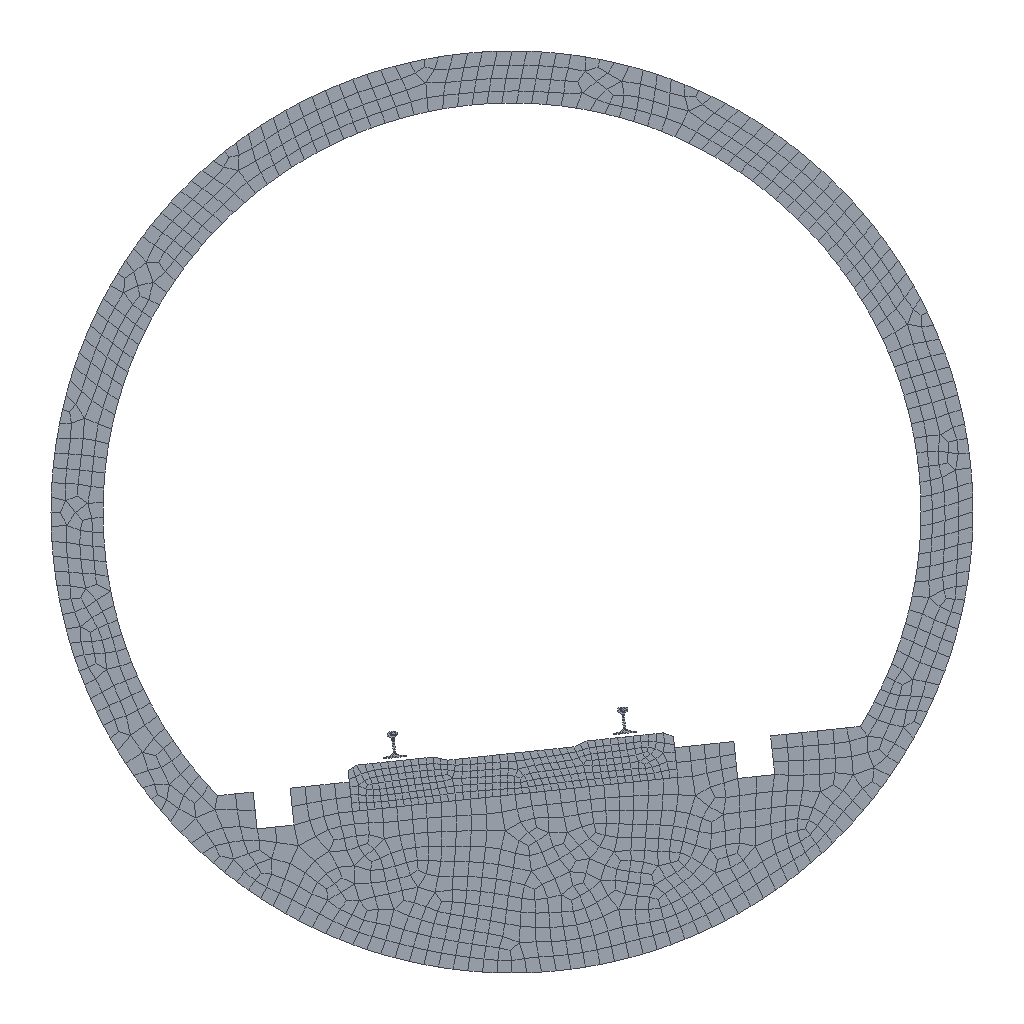Simulation study | abaqus
Set-up summary:
category,name,step,type,value,unit,region
solver,abaqus
solver,version,,,Abaqus/Standard 2020
units,not stated in the deck,,not stated
analysis,deck,,transient,transient
load_step,Step-1,Step-1,transient
load_step,requested,,,1
mesh,nodes,,,1882
mesh,elements,,,1560
element_type,CPS4R,,plane,1560
load,load commands in deck,,count,2
bc,support commands in deck,,count,1
material,CONCRETE,,in results
material,GUIZHEN,,in results
material,STEEL,,in results
check,setup vs results,,match,"per instance, exact: element labels, types and connectivity; labels of the nodes the elements use; coordinates of those nodes at SINGLE_PRECISION in 3 of 4 instance(s)"
Abaqus input file, long lists of numbers shortened:
*Heading
** Job name: Job-1 Model name: Model-1
** Generated by: Abaqus/CAE 2020
*Preprint, echo=NO, model=NO, history=NO, contact=NO
**
** PARTS
**
*Part, name=guizhen
*Node
      1,       -1037.,         913.
      2,       -1098.,        882.5
** (334 more lines like these left out)
*Element, type=CPS4R
  1, 331,  99,   1,  11
  2, 219, 261, 122, 120
** (284 more lines like these left out)
*Nset, nset=Set-1, generate
   1,  336,    1
*Elset, elset=Set-1, generate
   1,  286,    1
*Nset, nset=Set-2, generate
   1,  336,    1
*Elset, elset=Set-2, generate
   1,  286,    1
** Section: Section-3
*Solid Section, elset=Set-2, material=guizhen
,
*End Part
**
*Part, name=rail
*Node
      1,    -406.188,     360.812
      2,    -406.188,       364.75
** (159 more lines like these left out)
*Element, type=CPS4R
  1,  47,  48, 116, 117
  2,   3,   4,  97, 122
** (117 more lines like these left out)
*Nset, nset=Set-1, generate
   1,  161,    1
*Elset, elset=Set-1, generate
   1,  119,    1
*Nset, nset=Set-2, generate
   1,  161,    1
*Elset, elset=Set-2, generate
   1,  119,    1
** Section: Section-2
*Solid Section, elset=Set-2, material=steel
,
*End Part
**
*Part, name=structure
*Node
      1,   2478.045,  -1192.389
      2,   2554.355,  -1018.71
** (1222 more lines like these left out)
*Element, type=CPS4R
   1,  608,  582,  815,  240
   2,  553,  847, 1170,  239
** (1034 more lines like these left out)
*Nset, nset=Set-1, generate
    1,  1224,     1
*Elset, elset=Set-1, generate
    1,  1036,     1
*Nset, nset=Set-2, generate
    1,  1224,     1
*Elset, elset=Set-2, generate
    1,  1036,     1
** Section: Section-1
*Solid Section, elset=Set-2, material=concrete
,
*End Part
**
**
** ASSEMBLY
**
*Assembly, name=Assembly
**
*Instance, name=guizhen-1, part=guizhen
7804.25, -2501.585,           0.
7804.25, -2501.585,           0., 7804.25, -2501.585, 1., 6.
*End Instance
**
*Instance, name=rail-1, part=rail
7354.92, -1851.68,           0.
7354.92, -1851.68,           0., 7354.92, -1851.68, 1., 6.
*End Instance
**
*Instance, name=structure-1, part=structure
       7720.,           0.,           0.
*End Instance
**
*Instance, name=rail-1-lin-2-1, part=rail
8901.899, -1689.086,           0.
8901.899, -1689.086,           0., 8901.899, -1689.086, 1., 6.
*End Instance
**
*Node
      1,   6935.326,  -1674.883,           0.
*Node
      2,   6871.67,  -1648.302,           0.
*Node
      3,   6993.064,  -1635.542,           0.
*Node
      4,   8482.305,  -1512.289,           0.
*Node
      5,   8418.649,  -1485.708,           0.
*Node
      6,   8540.043,  -1472.948,           0.
*Node
      7,   8422.305,  -1518.289,           0.
*Node
      8,   8542.305,  -1506.289,           0.
*Node
      9,   6995.326,  -1667.883,           0.
*Node
     10,   6875.326,  -1680.883,           0.
*Node
     11,   6930.74,  -1474.075,           0.
*Node
     12,   8446.34,  -1314.779,           0.
*Nset, nset=Set-12
  2,  3,  5,  6,  7,  8,  9, 10
*Nset, nset=Set-13, instance=structure-1
  71,  72,  73,  74,  75,  76,  77,  78,  79,  80,  81,  82,  83,  84,  85,  86
  87,  88,  89,  90,  91,  92,  93,  94,  95,  96,  97,  98,  99, 100, 101, 102
** (11 more lines like these left out)
*Elset, elset=Set-13, instance=structure-1
  11,  12,  13,  19,  20,  46,  49,  58,  59,  65,  66,  67,  70,  71,  75,  76
 130, 131, 133, 138, 139, 146, 147, 148, 153, 167, 168, 169, 178, 181, 182, 183
** (11 more lines like these left out)
*Nset, nset=Set-14, instance=rail-1
 36,
*Nset, nset=Set-15, instance=rail-1
 36,
*Nset, nset=Set-16, instance=rail-1
 36,
*Nset, nset=Set-17
 11,
*Nset, nset=Set-18, generate
  7,  10,   1
*Nset, nset=Set-22
 2, 3
*Nset, nset=Set-23
 2, 3, 5, 6
*Nset, nset=Set-25
 12,
*Nset, nset=m_Set-13, instance=rail-1
 36,
*Nset, nset=m_Set-15
 11,
*Nset, nset=m_Set-18
 2,
*Nset, nset=m_Set-19
 3,
*Nset, nset=m_Set-20
 5,
*Nset, nset=m_Set-21
 6,
*Nset, nset=m_Set-24
 12,
*Nset, nset=m_Set-26
  9, 10
*Nset, nset=m_Set-27
 7, 8
*Nset, nset=m_Set-28
 10,
*Nset, nset=m_Set-29
 9,
*Nset, nset=m_Set-30
 7,
*Nset, nset=m_Set-31
 8,
*Nset, nset=m_Set-32
 10,
*Nset, nset=m_Set-33
 9,
*Nset, nset=m_Set-34
 7,
*Nset, nset=m_Set-35
 8,
*Elset, elset=_m_Surf-1_S4, internal, instance=structure-1
  26,  28,  36, 100, 418, 419
*Elset, elset=_m_Surf-1_S3, internal, instance=structure-1
 29, 39
*Elset, elset=_m_Surf-1_S2, internal, instance=structure-1
  41,  54, 109, 119, 123, 124, 322, 415, 416, 417, 733, 734, 735, 736, 737, 745
 746, 866
*Surface, type=ELEMENT, name=m_Surf-1
_m_Surf-1_S4, S4
_m_Surf-1_S3, S3
_m_Surf-1_S2, S2
*Elset, elset=_m_Surf-3_S4, internal, instance=structure-1
  26,  28,  36, 100, 418, 419
*Elset, elset=_m_Surf-3_S3, internal, instance=structure-1
 29, 39
*Elset, elset=_m_Surf-3_S2, internal, instance=structure-1
  41,  54, 109, 119, 123, 124, 322, 415, 416, 417, 733, 734, 735, 736, 737, 745
 746, 866
*Surface, type=ELEMENT, name=m_Surf-3
_m_Surf-3_S4, S4
_m_Surf-3_S3, S3
_m_Surf-3_S2, S2
*Elset, elset=_m_Surf-5_S1, internal, instance=rail-1-lin-2-1
  6,  8, 10, 15, 54, 91
*Elset, elset=_m_Surf-5_S4, internal, instance=rail-1-lin-2-1
  7, 13, 52
*Elset, elset=_m_Surf-5_S3, internal, instance=rail-1-lin-2-1
   9,  50,  90,  93, 112
*Elset, elset=_m_Surf-5_S2, internal, instance=rail-1-lin-2-1
  46,  66, 106
*Surface, type=ELEMENT, name=m_Surf-5
_m_Surf-5_S1, S1
_m_Surf-5_S4, S4
_m_Surf-5_S2, S2
_m_Surf-5_S3, S3
*Elset, elset=_m_Surf-7_S1, internal, instance=rail-1
  6,  8, 10, 15, 54, 91
*Elset, elset=_m_Surf-7_S4, internal, instance=rail-1
  7, 13, 52
*Elset, elset=_m_Surf-7_S3, internal, instance=rail-1
   9,  50,  90,  93, 112
*Elset, elset=_m_Surf-7_S2, internal, instance=rail-1
  46,  66, 106
*Surface, type=ELEMENT, name=m_Surf-7
_m_Surf-7_S1, S1
_m_Surf-7_S4, S4
_m_Surf-7_S2, S2
_m_Surf-7_S3, S3
*Elset, elset=_m_Surf-9_S2, internal, instance=guizhen-1
 9,
*Elset, elset=_m_Surf-9_S1, internal, instance=guizhen-1
 13,
*Elset, elset=_m_Surf-9_S3, internal, instance=guizhen-1
  92, 285
*Elset, elset=_m_Surf-9_S4, internal, instance=guizhen-1
 117,
*Surface, type=ELEMENT, name=m_Surf-9
_m_Surf-9_S2, S2
_m_Surf-9_S1, S1
_m_Surf-9_S4, S4
_m_Surf-9_S3, S3
*Elset, elset=_m_Surf-11_S4, internal, instance=guizhen-1
  11,  12,  18,  22,  23,  35,  37,  40,  42,  49,  51,  54,  62,  70,  74,  79
  83,  89,  91,  95,  97,  99, 108, 118, 126, 129
*Elset, elset=_m_Surf-11_S2, internal, instance=guizhen-1
  13,  16,  24,  30,  43,  47,  53,  55, 101, 102, 106, 110, 111, 112, 120, 121
 124, 128
*Surface, type=ELEMENT, name=m_Surf-11
_m_Surf-11_S4, S4
_m_Surf-11_S2, S2
*Elset, elset=_m_Surf-13_S3, internal, instance=guizhen-1
 55,
*Elset, elset=_m_Surf-13_S1, internal, instance=guizhen-1
 132, 133, 238
*Elset, elset=_m_Surf-13_S2, internal, instance=guizhen-1
 279,
*Surface, type=ELEMENT, name=m_Surf-13
_m_Surf-13_S3, S3
_m_Surf-13_S1, S1
_m_Surf-13_S2, S2
*Elset, elset=_m_Surf-20_S4, internal, instance=structure-1
  26,  28,  36, 100, 418, 419
*Elset, elset=_m_Surf-20_S3, internal, instance=structure-1
 29, 39
*Elset, elset=_m_Surf-20_S2, internal, instance=structure-1
  41,  54, 109, 119, 123, 124, 322, 415, 416, 417, 733, 734, 735, 736, 737, 745
 746, 866
*Surface, type=ELEMENT, name=m_Surf-20
_m_Surf-20_S4, S4
_m_Surf-20_S3, S3
_m_Surf-20_S2, S2
*Elset, elset=_s_Surf-1_S2, internal, instance=guizhen-1
   9, 279
*Elset, elset=_s_Surf-1_S1, internal, instance=guizhen-1
  13, 132, 133, 238
*Elset, elset=_s_Surf-1_S3, internal, instance=guizhen-1
  55,  92, 285
*Elset, elset=_s_Surf-1_S4, internal, instance=guizhen-1
 117,
*Surface, type=ELEMENT, name=s_Surf-1
_s_Surf-1_S2, S2
_s_Surf-1_S1, S1
_s_Surf-1_S4, S4
_s_Surf-1_S3, S3
*Elset, elset=_s_Surf-3_S2, internal, instance=guizhen-1
   9,  13,  16,  24,  30,  43,  47,  53,  55, 101, 102, 106, 110, 111, 112, 120
 121, 124, 128, 279
*Elset, elset=_s_Surf-3_S1, internal, instance=guizhen-1
  13, 132, 133, 238
*Elset, elset=_s_Surf-3_S3, internal, instance=guizhen-1
  55,  92, 285
*Elset, elset=_s_Surf-3_S4, internal, instance=guizhen-1
  11,  12,  18,  22,  23,  35,  37,  40,  42,  49,  51,  54,  62,  70,  74,  79
  83,  89,  91,  95,  97,  99, 108, 117, 118, 126, 129
*Surface, type=ELEMENT, name=s_Surf-3
_s_Surf-3_S2, S2
_s_Surf-3_S1, S1
_s_Surf-3_S4, S4
_s_Surf-3_S3, S3
*Elset, elset=_s_Surf-5_S3, internal, instance=guizhen-1
   7,  46,  48,  58,  59,  63,  66, 130
*Elset, elset=_s_Surf-5_S1, internal, instance=guizhen-1
  45, 153
*Surface, type=ELEMENT, name=s_Surf-5
_s_Surf-5_S3, S3
_s_Surf-5_S1, S1
*Elset, elset=_s_Surf-7_S3, internal, instance=guizhen-1
   4,  10,  15,  86,  90,  98, 158
*Elset, elset=_s_Surf-7_S1, internal, instance=guizhen-1
  85, 152, 160
*Surface, type=ELEMENT, name=s_Surf-7
_s_Surf-7_S3, S3
_s_Surf-7_S1, S1
*Elset, elset=_s_Surf-9_S4, internal, instance=structure-1
 28,
*Elset, elset=_s_Surf-9_S3, internal, instance=structure-1
 29,
*Surface, type=ELEMENT, name=s_Surf-9
_s_Surf-9_S4, S4
_s_Surf-9_S3, S3
*Elset, elset=_s_Surf-11_S4, internal, instance=structure-1
  26, 100, 418, 419
*Elset, elset=_s_Surf-11_S2, internal, instance=structure-1
  41,  54, 109, 119, 123, 124, 322, 415, 416, 417, 733, 734, 735, 736, 737, 745
 746, 866
*Surface, type=ELEMENT, name=s_Surf-11
_s_Surf-11_S4, S4
_s_Surf-11_S2, S2
*Elset, elset=_s_Surf-13_S4, internal, instance=structure-1
 36,
*Elset, elset=_s_Surf-13_S3, internal, instance=structure-1
 39,
*Surface, type=ELEMENT, name=s_Surf-13
_s_Surf-13_S4, S4
_s_Surf-13_S3, S3
*Elset, elset=_s_Surf-15_S2, internal, instance=rail-1
 30, 31, 84
*Elset, elset=_s_Surf-15_S1, internal, instance=rail-1
 35, 82
*Elset, elset=_s_Surf-15_S3, internal, instance=rail-1
 95,
*Surface, type=ELEMENT, name=s_Surf-15
_s_Surf-15_S2, S2
_s_Surf-15_S1, S1
_s_Surf-15_S3, S3
*Elset, elset=_s_Surf-16_S3, internal, instance=rail-1
 73, 74
*Elset, elset=_s_Surf-16_S1, internal, instance=rail-1
  14,  44, 113
*Elset, elset=_s_Surf-16_S4, internal, instance=rail-1
  14, 114
*Elset, elset=_s_Surf-16_S2, internal, instance=rail-1
 67,
*Surface, type=ELEMENT, name=s_Surf-16
_s_Surf-16_S3, S3
_s_Surf-16_S1, S1
_s_Surf-16_S4, S4
_s_Surf-16_S2, S2
*Elset, elset=_s_Surf-17_S1, internal, instance=rail-1
 102,
*Elset, elset=_s_Surf-17_S4, internal, instance=rail-1
  12,  56, 103
*Elset, elset=_s_Surf-17_S2, internal, instance=rail-1
 11, 57, 70
*Surface, type=ELEMENT, name=s_Surf-17
_s_Surf-17_S1, S1
_s_Surf-17_S4, S4
_s_Surf-17_S2, S2
*Elset, elset=_s_Surf-18_S3, internal, instance=rail-1-lin-2-1
 73, 74
*Elset, elset=_s_Surf-18_S1, internal, instance=rail-1-lin-2-1
  14,  44, 113
*Elset, elset=_s_Surf-18_S4, internal, instance=rail-1-lin-2-1
  14, 114
*Elset, elset=_s_Surf-18_S2, internal, instance=rail-1-lin-2-1
 67,
*Surface, type=ELEMENT, name=s_Surf-18
_s_Surf-18_S3, S3
_s_Surf-18_S1, S1
_s_Surf-18_S4, S4
_s_Surf-18_S2, S2
*Elset, elset=_s_Surf-19_S1, internal, instance=rail-1-lin-2-1
 102,
*Elset, elset=_s_Surf-19_S4, internal, instance=rail-1-lin-2-1
  12,  56, 103
*Elset, elset=_s_Surf-19_S2, internal, instance=rail-1-lin-2-1
 11, 57, 70
*Surface, type=ELEMENT, name=s_Surf-19
_s_Surf-19_S1, S1
_s_Surf-19_S4, S4
_s_Surf-19_S2, S2
*Elset, elset=_s_Surf-20_S2, internal, instance=guizhen-1
   9,  13,  16,  24,  30,  43,  47,  53,  55, 101, 102, 106, 110, 111, 112, 120
 121, 124, 128, 279
*Elset, elset=_s_Surf-20_S1, internal, instance=guizhen-1
  13, 132, 133, 238
*Elset, elset=_s_Surf-20_S3, internal, instance=guizhen-1
  55,  92, 285
*Elset, elset=_s_Surf-20_S4, internal, instance=guizhen-1
  11,  12,  18,  22,  23,  35,  37,  40,  42,  49,  51,  54,  62,  70,  74,  79
  83,  89,  91,  95,  97,  99, 108, 117, 118, 126, 129
*Surface, type=ELEMENT, name=s_Surf-20
_s_Surf-20_S2, S2
_s_Surf-20_S1, S1
_s_Surf-20_S4, S4
_s_Surf-20_S3, S3
*Elset, elset=_s_Surf-22_S2, internal, instance=rail-1-lin-2-1
 30, 83, 84
*Elset, elset=_s_Surf-22_S3, internal, instance=rail-1-lin-2-1
 64, 95
*Elset, elset=_s_Surf-22_S1, internal, instance=rail-1-lin-2-1
 115,
*Elset, elset=_s_Surf-22_S4, internal, instance=rail-1-lin-2-1
 25,
*Surface, type=ELEMENT, name=s_Surf-22
_s_Surf-22_S2, S2
_s_Surf-22_S3, S3
_s_Surf-22_S4, S4
_s_Surf-22_S1, S1
*Elset, elset=_s_Surf-23_S3, internal, instance=guizhen-1
   4,  10,  15,  86,  90,  98, 158
*Elset, elset=_s_Surf-23_S1, internal, instance=guizhen-1
  85, 152, 160
*Surface, type=ELEMENT, name=s_Surf-23
_s_Surf-23_S3, S3
_s_Surf-23_S1, S1
*Elset, elset=_s_Surf-24_S3, internal, instance=guizhen-1
   7,  46,  48,  58,  59,  63,  66, 130
*Elset, elset=_s_Surf-24_S1, internal, instance=guizhen-1
  45, 153
*Surface, type=ELEMENT, name=s_Surf-24
_s_Surf-24_S3, S3
_s_Surf-24_S1, S1
*Elset, elset=_s_Surf-25_S3, internal, instance=guizhen-1
   4,  10,  15,  86,  90,  98, 158
*Elset, elset=_s_Surf-25_S1, internal, instance=guizhen-1
  85, 152, 160
*Surface, type=ELEMENT, name=s_Surf-25
_s_Surf-25_S3, S3
_s_Surf-25_S1, S1
*Elset, elset=_s_Surf-26_S3, internal, instance=guizhen-1
   7,  46,  48,  58,  59,  63,  66, 130
*Elset, elset=_s_Surf-26_S1, internal, instance=guizhen-1
  45, 153
*Surface, type=ELEMENT, name=s_Surf-26
_s_Surf-26_S3, S3
_s_Surf-26_S1, S1
*Elset, elset=_s_Surf-27_S3, internal, instance=guizhen-1
   7,  46,  48,  58,  59,  63,  66, 130
*Elset, elset=_s_Surf-27_S1, internal, instance=guizhen-1
  45, 153
*Surface, type=ELEMENT, name=s_Surf-27
_s_Surf-27_S3, S3
_s_Surf-27_S1, S1
*Elset, elset=_s_Surf-28_S3, internal, instance=guizhen-1
 1,
*Elset, elset=_s_Surf-28_S2, internal, instance=guizhen-1
 285,
*Surface, type=ELEMENT, name=s_Surf-28
_s_Surf-28_S3, S3
_s_Surf-28_S2, S2
*Elset, elset=_s_Surf-29_S3, internal, instance=guizhen-1
 21, 84
*Surface, type=ELEMENT, name=s_Surf-29
_s_Surf-29_S3, S3
*Elset, elset=_s_Surf-30_S1, internal, instance=guizhen-1
 8,
*Elset, elset=_s_Surf-30_S3, internal, instance=guizhen-1
 68,
*Surface, type=ELEMENT, name=s_Surf-30
_s_Surf-30_S1, S1
_s_Surf-30_S3, S3
*Elset, elset=_s_Surf-31_S3, internal, instance=guizhen-1
 279,
*Surface, type=ELEMENT, name=s_Surf-31
_s_Surf-31_S3, S3
** Constraint: Constraint-1
*Tie, name=Constraint-1, adjust=yes
s_Surf-3, m_Surf-3
** Constraint: Constraint-2
*Coupling, constraint name=Constraint-2, ref node=m_Set-15, surface=s_Surf-15
*Kinematic
** Constraint: Constraint-3
*Coupling, constraint name=Constraint-3, ref node=m_Set-18, surface=s_Surf-16
*Kinematic
** Constraint: Constraint-4
*Coupling, constraint name=Constraint-4, ref node=m_Set-19, surface=s_Surf-17
*Kinematic
** Constraint: Constraint-5
*Coupling, constraint name=Constraint-5, ref node=m_Set-20, surface=s_Surf-18
*Kinematic
** Constraint: Constraint-6
*Coupling, constraint name=Constraint-6, ref node=m_Set-21, surface=s_Surf-19
*Kinematic
** Constraint: Constraint-7
*Coupling, constraint name=Constraint-7, ref node=m_Set-24, surface=s_Surf-22
*Kinematic
** Constraint: Constraint-12
*Coupling, constraint name=Constraint-12, ref node=m_Set-32, surface=s_Surf-28
*Kinematic
** Constraint: Constraint-13
*Coupling, constraint name=Constraint-13, ref node=m_Set-33, surface=s_Surf-29
*Kinematic
** Constraint: Constraint-14
*Coupling, constraint name=Constraint-14, ref node=m_Set-34, surface=s_Surf-30
*Kinematic
** Constraint: Constraint-15
*Coupling, constraint name=Constraint-15, ref node=m_Set-35, surface=s_Surf-31
*Kinematic
*Element, type=MASS, elset=Set-23_Inertia-1_
1, 2
2, 3
** (2 more lines like these left out)
*Mass, elset=Set-23_Inertia-1_
10.,
*Spring, elset=Springs/Dashpots-1-spring
60000.
*Element, type=SpringA, elset=Springs/Dashpots-1-spring
5, 2, 10
6, 3, 9
** (2 more lines like these left out)
*End Assembly
*Amplitude, name=Amp-1
             0.,              0.,     0.0001042,              0.,     0.0002084,              0.,     0.0003126,              0.
    0.0004168,              0.,     0.000521,              0.,     0.0006252,              0.,     0.0007294,              0.
    0.0008336,              0.,     0.0009378,              0.,     0.001042,              0.,     0.001146,              0.
    0.00125,              0.,      0.001355,              0.,     0.001459,              0.,     0.001563,              0.
    0.001667,              0.,     0.001771,     4.983,     0.001876,              0.,     0.00198,              0.
    0.002084,              0.,     0.002188,              0.,     0.002292,              0.,     0.002397,              0.
    0.002501,              0.,     0.002605,              0.,      0.002709,              0.,     0.002813,              0.
    0.002918,              0.,     0.003022,              0.,     0.003126,              0.,     0.00323,              0.
    0.003334,              0.,     0.003439,              0.,     0.003543,              0.,     0.003647,              0.
    0.003751,              0.,     0.003855,              0.,     0.00396,              0.,      0.004064,              0.
    0.004168,              0.,     0.004272,              0.,     0.004376,              0.,     0.004481,              0.
    0.004585,              0.,     0.004689,     30.845,     0.004793,              0.,     0.004897,              0.
    0.005002,              0.,     0.005106,              0.,     0.00521,              0.,     0.005314,              0.
     0.005418,              0.,     0.005523,              0.,     0.005627,              0.,     0.005731,              0.
    0.005835,              0.,     0.005939,              0.,     0.006044,              0.,     0.006148,              0.
    0.006252,              0.,     0.006356,              0.,     0.00646,     1.132,     0.006565,              0.
    0.006669,              0.,      0.006773,              0.,     0.006877,              0.,     0.006981,              0.
    0.007086,              0.,     0.00719,     1.579,     0.007294,              0.,     0.007398,              0.
    0.007502,              0.,     0.007607,      1.579,     0.007711,     5.487,     0.007815,              0.
    0.007919,              0.,     0.008023,     0.5184,      0.008128,     0.3864,     0.008232,     0.3959
    0.008336,     1.472,     0.00844,     0.1397,     0.008544,     1.95,     0.008649,     0.01693
    0.008753,     1.235,     0.008857,     0.6286,     0.008961,     0.34,     0.009065,      1.358
    0.00917,     0.3606,     0.009274,     1.281,     0.009378,     0.3096,      0.009482,     1.376
    0.009586,     0.4285,     0.009691,     0.7766,     0.009795,     0.9554,     0.009899,     0.5412
    0.01,     1.006,     0.01011,     0.5866,     0.01021,     1.092,     0.01032,     0.5136
    0.01042,     1.052,     0.01052,     0.7341,     0.01063,     0.7525,     0.01073,     0.8903
     0.01084,     0.724,     0.01094,     0.8668,     0.01105,     0.6484,     0.01115,      0.9454
    0.01125,     0.6244,     0.01136,     0.8135,     0.01146,     0.7672,     0.01157,     0.6908
    0.01167,     0.7609,     0.01177,     0.6851,     0.01188,     0.7993,     0.01198,       0.6252
    0.01209,     0.8602,      0.01219,     0.6965,     0.0123,     0.7902,     0.0124,     0.7834
    0.0125,      0.7767,     0.01261,     0.79,     0.01271,     0.7511,     0.01282,     0.8588
    0.01292,     0.7269,     0.01302,     0.8595,     0.01313,     0.7674,     0.01323,     0.8312
    0.01334,      0.7565,     0.01344,     0.815,       0.01355,     0.7644,     0.01365,     0.7777
    0.01375,     0.8086,     0.01386,     0.7827,     0.01396,     0.8265,     0.01407,      0.79
    0.01417,      0.848,     0.01428,     0.8046,     0.01438,     0.8434,     0.01448,      0.8076
    0.01459,     0.8435,     0.01469,     0.8179,     0.0148,     0.8458,      0.0149,       0.8107
    0.015,     0.8199,     0.01511,     0.8019,     0.01521,     0.7867,     0.01532,     0.7737
    0.01542,     0.7759,     0.01553,     0.7753,     0.01563,     0.7813,     0.01573,      0.7905
    0.01584,     0.7859,     0.01594,     0.797,     0.01605,      0.8029,      0.01615,     0.8192
     0.01626,     0.8216,     0.01636,     0.8422,     0.01646,     0.8465,     0.01657,     0.8628
** (1960 more lines like these left out)
**
** MATERIALS
**
*Material, name=concrete
*Density
 2.5e-09,
*Elastic
30000., 0.2
*Material, name=guizhen
*Density
 2.5e-09,
*Elastic
36000., 0.2
*Material, name=steel
*Density
 7.8e-09,
*Elastic
210000., 0.3
**
** INTERACTION PROPERTIES
**
*Surface Interaction, name=IntProp-1
1.,
*Friction, slip tolerance=0.005
 0.1,
*Surface Behavior, pressure-overclosure=HARD
*Surface Interaction, name=IntProp-2
1.,
*Friction, rough
*Surface Behavior, pressure-overclosure=HARD
** ----------------------------------------------------------------
**
** STEP: Step-1
**
*Step, name=Step-1, nlgeom=YES, inc=100000
*Dynamic
0.01,1.,1e-05
**
** BOUNDARY CONDITIONS
**
** Name: BC-1 Type: 对称/反对称/完全固定
*Boundary
Set-13, ENCASTRE
**
** LOADS
**
** Name: Load-1   Type: Concentrated force
*Cload, amplitude=Amp-1
Set-17, 2, -999.587
** Name: Load-1-Copy   Type: Concentrated force
*Cload, amplitude=Amp-1
Set-25, 2, -999.587
**
** OUTPUT REQUESTS
**
*Restart, write, number interval=1, time marks=NO
**
** FIELD OUTPUT: F-Output-1
**
*Output, field, frequency=1
*Node Output
A, RF, RT, U, V
*Element Output, directions=YES
E, LE, MISES, MISESMAX, PEEQ, S
*Contact Output
CSTRESS,
**
** HISTORY OUTPUT: H-Output-1
**
*Output, history, variable=PRESELECT, number interval=200, time marks=NO
*End Step
Results summary:
result,step,,completed,increments=190 time=1.0/1.0
result,analysis,,,transient
result,last_loadstep,,,1
result,primary field,,,U
result,reaction total,,FX,-320.558,model units
result,reaction total,,FY,1859.691,model units
result,reaction total,,FZ,0.0,model units